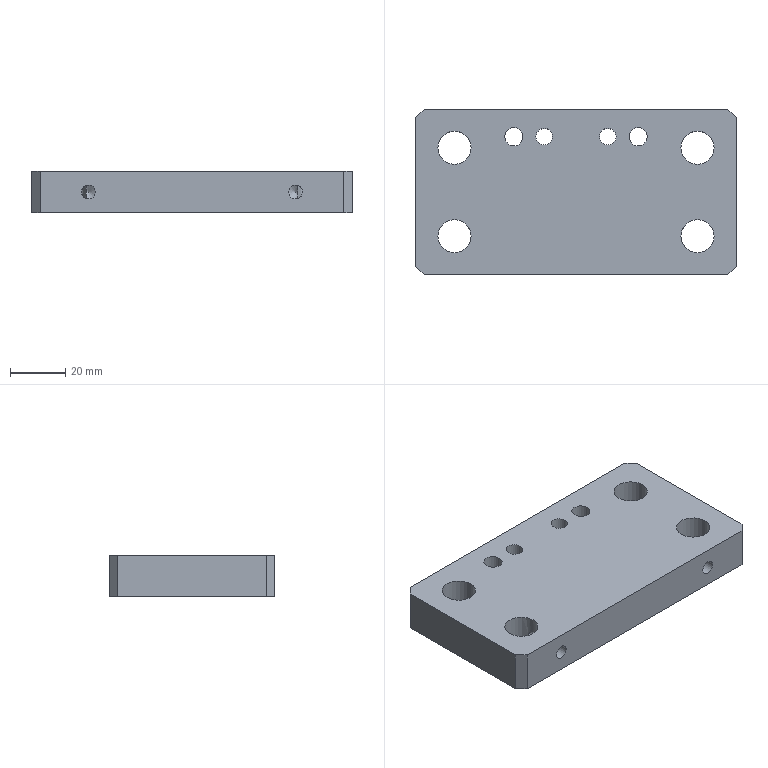Part | NX | features BREP 1 | 1 solid | 29 faces | box 116 x 60 x 15 mm | volume 93839 mm3 | cylinder 14 | plane 12 | cone 3 | commonest cylinder face diameters 5 x4 12 x4 6 x2 6.6 x2 11 x2
STEP:
#1=CARTESIAN_POINT('',(58.,0.,-5.));
#2=VERTEX_POINT('',#1);
#3=CARTESIAN_POINT('',(58.,0.,-7.5));
#4=DIRECTION('',(-1.,0.,0.));
#5=DIRECTION('',(0.,0.,1.));
#6=AXIS2_PLACEMENT_3D('',#3,#4,#5);
#7=CIRCLE('',#6,2.5);
#8=EDGE_CURVE('',#2,#2,#7,.T.);
#9=ORIENTED_EDGE('',*,*,#8,.T.);
#10=EDGE_LOOP('',(#9));
#11=FACE_BOUND('',#10,.T.);
#12=CARTESIAN_POINT('',(58.,-27.,0.));
#13=VERTEX_POINT('',#12);
#14=CARTESIAN_POINT('',(58.,27.,0.));
#15=VERTEX_POINT('',#14);
#16=CARTESIAN_POINT('',(58.,30.,0.));
#17=DIRECTION('',(0.,1.,0.));
#18=VECTOR('',#17,1000.);
#19=LINE('',#16,#18);
#20=EDGE_CURVE('',#13,#15,#19,.T.);
#21=ORIENTED_EDGE('',*,*,#20,.F.);
#22=CARTESIAN_POINT('',(58.,-27.,-15.));
#23=VERTEX_POINT('',#22);
#24=CARTESIAN_POINT('',(58.,-27.,-15.));
#25=DIRECTION('',(0.,0.,1.));
#26=VECTOR('',#25,1000.);
#27=LINE('',#24,#26);
#28=EDGE_CURVE('',#23,#13,#27,.T.);
#29=ORIENTED_EDGE('',*,*,#28,.F.);
#30=CARTESIAN_POINT('',(58.,27.,-15.));
#31=VERTEX_POINT('',#30);
#32=CARTESIAN_POINT('',(58.,30.,-15.));
#33=DIRECTION('',(0.,1.,0.));
#34=VECTOR('',#33,1000.);
#35=LINE('',#32,#34);
#36=EDGE_CURVE('',#23,#31,#35,.T.);
#37=ORIENTED_EDGE('',*,*,#36,.T.);
#38=CARTESIAN_POINT('',(58.,27.,-15.));
#39=DIRECTION('',(0.,0.,-1.));
#40=VECTOR('',#39,1000.);
#41=LINE('',#38,#40);
#42=EDGE_CURVE('',#15,#31,#41,.T.);
#43=ORIENTED_EDGE('',*,*,#42,.F.);
#44=EDGE_LOOP('',(#21,#29,#37,#43));
#45=FACE_BOUND('',#44,.T.);
#46=CARTESIAN_POINT('',(58.,30.,-15.));
#47=DIRECTION('',(-1.,0.,0.));
#48=DIRECTION('',(0.,1.,0.));
#49=AXIS2_PLACEMENT_3D('',#46,#47,#48);
#50=PLANE('',#49);
#51=ADVANCED_FACE('',(#11,#45),#50,.F.);
#52=CARTESIAN_POINT('',(55.,30.,-15.));
#53=VERTEX_POINT('',#52);
#54=CARTESIAN_POINT('',(-55.,30.,-15.));
#55=VERTEX_POINT('',#54);
#56=CARTESIAN_POINT('',(-58.,30.,-15.));
#57=DIRECTION('',(-1.,0.,0.));
#58=VECTOR('',#57,1000.);
#59=LINE('',#56,#58);
#60=EDGE_CURVE('',#53,#55,#59,.T.);
#61=ORIENTED_EDGE('',*,*,#60,.T.);
#62=CARTESIAN_POINT('',(-55.,30.,0.));
#63=VERTEX_POINT('',#62);
#64=CARTESIAN_POINT('',(-55.,30.,-15.));
#65=DIRECTION('',(0.,0.,-1.));
#66=VECTOR('',#65,1000.);
#67=LINE('',#64,#66);
#68=EDGE_CURVE('',#63,#55,#67,.T.);
#69=ORIENTED_EDGE('',*,*,#68,.F.);
#70=CARTESIAN_POINT('',(55.,30.,0.));
#71=VERTEX_POINT('',#70);
#72=CARTESIAN_POINT('',(-58.,30.,0.));
#73=DIRECTION('',(-1.,0.,0.));
#74=VECTOR('',#73,1000.);
#75=LINE('',#72,#74);
#76=EDGE_CURVE('',#71,#63,#75,.T.);
#77=ORIENTED_EDGE('',*,*,#76,.F.);
#78=CARTESIAN_POINT('',(55.,30.,-15.));
#79=DIRECTION('',(0.,0.,1.));
#80=VECTOR('',#79,1000.);
#81=LINE('',#78,#80);
#82=EDGE_CURVE('',#53,#71,#81,.T.);
#83=ORIENTED_EDGE('',*,*,#82,.F.);
#84=EDGE_LOOP('',(#61,#69,#77,#83));
#85=FACE_BOUND('',#84,.T.);
#86=CARTESIAN_POINT('',(-58.,30.,-15.));
#87=DIRECTION('',(0.,-1.,0.));
#88=DIRECTION('',(0.,0.,-1.));
#89=AXIS2_PLACEMENT_3D('',#86,#87,#88);
#90=PLANE('',#89);
#91=ADVANCED_FACE('',(#85),#90,.F.);
#92=CARTESIAN_POINT('',(-58.,27.,-15.));
#93=VERTEX_POINT('',#92);
#94=CARTESIAN_POINT('',(-58.,-27.,-15.));
#95=VERTEX_POINT('',#94);
#96=CARTESIAN_POINT('',(-58.,30.,-15.));
#97=DIRECTION('',(0.,-1.,0.));
#98=VECTOR('',#97,1000.);
#99=LINE('',#96,#98);
#100=EDGE_CURVE('',#93,#95,#99,.T.);
#101=ORIENTED_EDGE('',*,*,#100,.T.);
#102=CARTESIAN_POINT('',(-58.,-27.,0.));
#103=VERTEX_POINT('',#102);
#104=CARTESIAN_POINT('',(-58.,-27.,-15.));
#105=DIRECTION('',(0.,0.,-1.));
#106=VECTOR('',#105,1000.);
#107=LINE('',#104,#106);
#108=EDGE_CURVE('',#103,#95,#107,.T.);
#109=ORIENTED_EDGE('',*,*,#108,.F.);
#110=CARTESIAN_POINT('',(-58.,27.,0.));
#111=VERTEX_POINT('',#110);
#112=CARTESIAN_POINT('',(-58.,30.,0.));
#113=DIRECTION('',(0.,-1.,0.));
#114=VECTOR('',#113,1000.);
#115=LINE('',#112,#114);
#116=EDGE_CURVE('',#111,#103,#115,.T.);
#117=ORIENTED_EDGE('',*,*,#116,.F.);
#118=CARTESIAN_POINT('',(-58.,27.,-15.));
#119=DIRECTION('',(0.,0.,1.));
#120=VECTOR('',#119,1000.);
#121=LINE('',#118,#120);
#122=EDGE_CURVE('',#93,#111,#121,.T.);
#123=ORIENTED_EDGE('',*,*,#122,.F.);
#124=EDGE_LOOP('',(#101,#109,#117,#123));
#125=FACE_BOUND('',#124,.T.);
#126=CARTESIAN_POINT('',(-58.,30.,-15.));
#127=DIRECTION('',(1.,0.,0.));
#128=DIRECTION('',(0.,-1.,0.));
#129=AXIS2_PLACEMENT_3D('',#126,#127,#128);
#130=PLANE('',#129);
#131=ADVANCED_FACE('',(#125),#130,.F.);
#132=CARTESIAN_POINT('',(37.5,-30.,-5.));
#133=VERTEX_POINT('',#132);
#134=CARTESIAN_POINT('',(37.5,-30.,-7.5));
#135=DIRECTION('',(0.,1.,0.));
#136=DIRECTION('',(0.,0.,1.));
#137=AXIS2_PLACEMENT_3D('',#134,#135,#136);
#138=CIRCLE('',#137,2.5);
#139=EDGE_CURVE('',#133,#133,#138,.T.);
#140=ORIENTED_EDGE('',*,*,#139,.T.);
#141=EDGE_LOOP('',(#140));
#142=FACE_BOUND('',#141,.T.);
#143=CARTESIAN_POINT('',(-37.5,-30.,-5.));
#144=VERTEX_POINT('',#143);
#145=CARTESIAN_POINT('',(-37.5,-30.,-7.5));
#146=DIRECTION('',(0.,1.,0.));
#147=DIRECTION('',(0.,0.,1.));
#148=AXIS2_PLACEMENT_3D('',#145,#146,#147);
#149=CIRCLE('',#148,2.5);
#150=EDGE_CURVE('',#144,#144,#149,.T.);
#151=ORIENTED_EDGE('',*,*,#150,.T.);
#152=EDGE_LOOP('',(#151));
#153=FACE_BOUND('',#152,.T.);
#154=CARTESIAN_POINT('',(-55.,-30.,0.));
#155=VERTEX_POINT('',#154);
#156=CARTESIAN_POINT('',(55.,-30.,0.));
#157=VERTEX_POINT('',#156);
#158=CARTESIAN_POINT('',(-58.,-30.,0.));
#159=DIRECTION('',(1.,0.,0.));
#160=VECTOR('',#159,1000.);
#161=LINE('',#158,#160);
#162=EDGE_CURVE('',#155,#157,#161,.T.);
#163=ORIENTED_EDGE('',*,*,#162,.F.);
#164=CARTESIAN_POINT('',(-55.,-30.,-15.));
#165=VERTEX_POINT('',#164);
#166=CARTESIAN_POINT('',(-55.,-30.,-15.));
#167=DIRECTION('',(0.,0.,1.));
#168=VECTOR('',#167,1000.);
#169=LINE('',#166,#168);
#170=EDGE_CURVE('',#165,#155,#169,.T.);
#171=ORIENTED_EDGE('',*,*,#170,.F.);
#172=CARTESIAN_POINT('',(55.,-30.,-15.));
#173=VERTEX_POINT('',#172);
#174=CARTESIAN_POINT('',(-58.,-30.,-15.));
#175=DIRECTION('',(1.,0.,0.));
#176=VECTOR('',#175,1000.);
#177=LINE('',#174,#176);
#178=EDGE_CURVE('',#165,#173,#177,.T.);
#179=ORIENTED_EDGE('',*,*,#178,.T.);
#180=CARTESIAN_POINT('',(55.,-30.,-15.));
#181=DIRECTION('',(0.,0.,-1.));
#182=VECTOR('',#181,1000.);
#183=LINE('',#180,#182);
#184=EDGE_CURVE('',#157,#173,#183,.T.);
#185=ORIENTED_EDGE('',*,*,#184,.F.);
#186=EDGE_LOOP('',(#163,#171,#179,#185));
#187=FACE_BOUND('',#186,.T.);
#188=CARTESIAN_POINT('',(-58.,-30.,-15.));
#189=DIRECTION('',(0.,1.,0.));
#190=DIRECTION('',(0.,0.,1.));
#191=AXIS2_PLACEMENT_3D('',#188,#189,#190);
#192=PLANE('',#191);
#193=ADVANCED_FACE('',(#142,#153,#187),#192,.F.);
#194=CARTESIAN_POINT('',(38.,16.,-15.));
#195=VERTEX_POINT('',#194);
#196=CARTESIAN_POINT('',(44.,16.,-15.));
#197=DIRECTION('',(0.,0.,-1.));
#198=DIRECTION('',(-1.,0.,0.));
#199=AXIS2_PLACEMENT_3D('',#196,#197,#198);
#200=CIRCLE('',#199,6.);
#201=EDGE_CURVE('',#195,#195,#200,.T.);
#202=ORIENTED_EDGE('',*,*,#201,.F.);
#203=EDGE_LOOP('',(#202));
#204=FACE_BOUND('',#203,.T.);
#205=CARTESIAN_POINT('',(38.,-16.,-15.));
#206=VERTEX_POINT('',#205);
#207=CARTESIAN_POINT('',(44.,-16.,-15.));
#208=DIRECTION('',(0.,0.,-1.));
#209=DIRECTION('',(-1.,0.,0.));
#210=AXIS2_PLACEMENT_3D('',#207,#208,#209);
#211=CIRCLE('',#210,6.);
#212=EDGE_CURVE('',#206,#206,#211,.T.);
#213=ORIENTED_EDGE('',*,*,#212,.F.);
#214=EDGE_LOOP('',(#213));
#215=FACE_BOUND('',#214,.T.);
#216=CARTESIAN_POINT('',(-50.,-16.,-15.));
#217=VERTEX_POINT('',#216);
#218=CARTESIAN_POINT('',(-44.,-16.,-15.));
#219=DIRECTION('',(0.,0.,-1.));
#220=DIRECTION('',(-1.,0.,0.));
#221=AXIS2_PLACEMENT_3D('',#218,#219,#220);
#222=CIRCLE('',#221,6.);
#223=EDGE_CURVE('',#217,#217,#222,.T.);
#224=ORIENTED_EDGE('',*,*,#223,.F.);
#225=EDGE_LOOP('',(#224));
#226=FACE_BOUND('',#225,.T.);
#227=CARTESIAN_POINT('',(-50.,16.,-15.));
#228=VERTEX_POINT('',#227);
#229=CARTESIAN_POINT('',(-44.,16.,-15.));
#230=DIRECTION('',(0.,0.,-1.));
#231=DIRECTION('',(-1.,0.,0.));
#232=AXIS2_PLACEMENT_3D('',#229,#230,#231);
#233=CIRCLE('',#232,6.);
#234=EDGE_CURVE('',#228,#228,#233,.T.);
#235=ORIENTED_EDGE('',*,*,#234,.F.);
#236=EDGE_LOOP('',(#235));
#237=FACE_BOUND('',#236,.T.);
#238=CARTESIAN_POINT('',(28.,20.,-15.));
#239=VERTEX_POINT('',#238);
#240=CARTESIAN_POINT('',(22.5,20.,-15.));
#241=DIRECTION('',(0.,0.,1.));
#242=DIRECTION('',(1.,0.,0.));
#243=AXIS2_PLACEMENT_3D('',#240,#241,#242);
#244=CIRCLE('',#243,5.5);
#245=EDGE_CURVE('',#239,#239,#244,.T.);
#246=ORIENTED_EDGE('',*,*,#245,.T.);
#247=EDGE_LOOP('',(#246));
#248=FACE_BOUND('',#247,.T.);
#249=CARTESIAN_POINT('',(-17.,20.,-15.));
#250=VERTEX_POINT('',#249);
#251=CARTESIAN_POINT('',(-22.5,20.,-15.));
#252=DIRECTION('',(0.,0.,1.));
#253=DIRECTION('',(1.,0.,0.));
#254=AXIS2_PLACEMENT_3D('',#251,#252,#253);
#255=CIRCLE('',#254,5.5);
#256=EDGE_CURVE('',#250,#250,#255,.T.);
#257=ORIENTED_EDGE('',*,*,#256,.T.);
#258=EDGE_LOOP('',(#257));
#259=FACE_BOUND('',#258,.T.);
#260=CARTESIAN_POINT('',(-14.5,20.,-15.));
#261=VERTEX_POINT('',#260);
#262=CARTESIAN_POINT('',(-11.5,20.,-15.));
#263=DIRECTION('',(0.,0.,-1.));
#264=DIRECTION('',(-1.,0.,0.));
#265=AXIS2_PLACEMENT_3D('',#262,#263,#264);
#266=CIRCLE('',#265,3.);
#267=EDGE_CURVE('',#261,#261,#266,.T.);
#268=ORIENTED_EDGE('',*,*,#267,.F.);
#269=EDGE_LOOP('',(#268));
#270=FACE_BOUND('',#269,.T.);
#271=CARTESIAN_POINT('',(8.5,20.,-15.));
#272=VERTEX_POINT('',#271);
#273=CARTESIAN_POINT('',(11.5,20.,-15.));
#274=DIRECTION('',(0.,0.,-1.));
#275=DIRECTION('',(-1.,0.,0.));
#276=AXIS2_PLACEMENT_3D('',#273,#274,#275);
#277=CIRCLE('',#276,3.);
#278=EDGE_CURVE('',#272,#272,#277,.T.);
#279=ORIENTED_EDGE('',*,*,#278,.F.);
#280=EDGE_LOOP('',(#279));
#281=FACE_BOUND('',#280,.T.);
#282=ORIENTED_EDGE('',*,*,#36,.F.);
#283=CARTESIAN_POINT('',(42.5,-42.5,-15.));
#284=DIRECTION('',(0.7071,0.7071,0.));
#285=VECTOR('',#284,1000.);
#286=LINE('',#283,#285);
#287=EDGE_CURVE('',#173,#23,#286,.T.);
#288=ORIENTED_EDGE('',*,*,#287,.F.);
#289=ORIENTED_EDGE('',*,*,#178,.F.);
#290=CARTESIAN_POINT('',(-42.5,-42.5,-15.));
#291=DIRECTION('',(0.7071,-0.7071,0.));
#292=VECTOR('',#291,1000.);
#293=LINE('',#290,#292);
#294=EDGE_CURVE('',#95,#165,#293,.T.);
#295=ORIENTED_EDGE('',*,*,#294,.F.);
#296=ORIENTED_EDGE('',*,*,#100,.F.);
#297=CARTESIAN_POINT('',(-42.5,42.5,-15.));
#298=DIRECTION('',(-0.7071,-0.7071,0.));
#299=VECTOR('',#298,1000.);
#300=LINE('',#297,#299);
#301=EDGE_CURVE('',#55,#93,#300,.T.);
#302=ORIENTED_EDGE('',*,*,#301,.F.);
#303=ORIENTED_EDGE('',*,*,#60,.F.);
#304=CARTESIAN_POINT('',(42.5,42.5,-15.));
#305=DIRECTION('',(-0.7071,0.7071,0.));
#306=VECTOR('',#305,1000.);
#307=LINE('',#304,#306);
#308=EDGE_CURVE('',#31,#53,#307,.T.);
#309=ORIENTED_EDGE('',*,*,#308,.F.);
#310=EDGE_LOOP('',(#282,#288,#289,#295,#296,#302,#303,#309));
#311=FACE_BOUND('',#310,.T.);
#312=CARTESIAN_POINT('',(0.,0.,-15.));
#313=DIRECTION('',(0.,0.,-1.));
#314=DIRECTION('',(-1.,0.,0.));
#315=AXIS2_PLACEMENT_3D('',#312,#313,#314);
#316=PLANE('',#315);
#317=ADVANCED_FACE('',(#204,#215,#226,#237,#248,#259,#270,#281,#311),#316,.T.);
#318=CARTESIAN_POINT('',(38.,16.,0.));
#319=VERTEX_POINT('',#318);
#320=CARTESIAN_POINT('',(44.,16.,0.));
#321=DIRECTION('',(0.,0.,-1.));
#322=DIRECTION('',(-1.,0.,0.));
#323=AXIS2_PLACEMENT_3D('',#320,#321,#322);
#324=CIRCLE('',#323,6.);
#325=EDGE_CURVE('',#319,#319,#324,.T.);
#326=ORIENTED_EDGE('',*,*,#325,.T.);
#327=EDGE_LOOP('',(#326));
#328=FACE_BOUND('',#327,.T.);
#329=CARTESIAN_POINT('',(38.,-16.,0.));
#330=VERTEX_POINT('',#329);
#331=CARTESIAN_POINT('',(44.,-16.,0.));
#332=DIRECTION('',(0.,0.,-1.));
#333=DIRECTION('',(-1.,0.,0.));
#334=AXIS2_PLACEMENT_3D('',#331,#332,#333);
#335=CIRCLE('',#334,6.);
#336=EDGE_CURVE('',#330,#330,#335,.T.);
#337=ORIENTED_EDGE('',*,*,#336,.T.);
#338=EDGE_LOOP('',(#337));
#339=FACE_BOUND('',#338,.T.);
#340=CARTESIAN_POINT('',(-50.,-16.,0.));
#341=VERTEX_POINT('',#340);
#342=CARTESIAN_POINT('',(-44.,-16.,0.));
#343=DIRECTION('',(0.,0.,-1.));
#344=DIRECTION('',(-1.,0.,0.));
#345=AXIS2_PLACEMENT_3D('',#342,#343,#344);
#346=CIRCLE('',#345,6.);
#347=EDGE_CURVE('',#341,#341,#346,.T.);
#348=ORIENTED_EDGE('',*,*,#347,.T.);
#349=EDGE_LOOP('',(#348));
#350=FACE_BOUND('',#349,.T.);
#351=CARTESIAN_POINT('',(-50.,16.,0.));
#352=VERTEX_POINT('',#351);
#353=CARTESIAN_POINT('',(-44.,16.,0.));
#354=DIRECTION('',(0.,0.,-1.));
#355=DIRECTION('',(-1.,0.,0.));
#356=AXIS2_PLACEMENT_3D('',#353,#354,#355);
#357=CIRCLE('',#356,6.);
#358=EDGE_CURVE('',#352,#352,#357,.T.);
#359=ORIENTED_EDGE('',*,*,#358,.T.);
#360=EDGE_LOOP('',(#359));
#361=FACE_BOUND('',#360,.T.);
#362=CARTESIAN_POINT('',(25.8,20.,0.));
#363=VERTEX_POINT('',#362);
#364=CARTESIAN_POINT('',(22.5,20.,0.));
#365=DIRECTION('',(0.,0.,1.));
#366=DIRECTION('',(1.,0.,0.));
#367=AXIS2_PLACEMENT_3D('',#364,#365,#366);
#368=CIRCLE('',#367,3.3);
#369=EDGE_CURVE('',#363,#363,#368,.T.);
#370=ORIENTED_EDGE('',*,*,#369,.F.);
#371=EDGE_LOOP('',(#370));
#372=FACE_BOUND('',#371,.T.);
#373=CARTESIAN_POINT('',(-19.2,20.,0.));
#374=VERTEX_POINT('',#373);
#375=CARTESIAN_POINT('',(-22.5,20.,0.));
#376=DIRECTION('',(0.,0.,1.));
#377=DIRECTION('',(1.,0.,0.));
#378=AXIS2_PLACEMENT_3D('',#375,#376,#377);
#379=CIRCLE('',#378,3.3);
#380=EDGE_CURVE('',#374,#374,#379,.T.);
#381=ORIENTED_EDGE('',*,*,#380,.F.);
#382=EDGE_LOOP('',(#381));
#383=FACE_BOUND('',#382,.T.);
#384=CARTESIAN_POINT('',(-14.5,20.,0.));
#385=VERTEX_POINT('',#384);
#386=CARTESIAN_POINT('',(-11.5,20.,0.));
#387=DIRECTION('',(0.,0.,-1.));
#388=DIRECTION('',(-1.,0.,0.));
#389=AXIS2_PLACEMENT_3D('',#386,#387,#388);
#390=CIRCLE('',#389,3.);
#391=EDGE_CURVE('',#385,#385,#390,.T.);
#392=ORIENTED_EDGE('',*,*,#391,.T.);
#393=EDGE_LOOP('',(#392));
#394=FACE_BOUND('',#393,.T.);
#395=CARTESIAN_POINT('',(8.5,20.,0.));
#396=VERTEX_POINT('',#395);
#397=CARTESIAN_POINT('',(11.5,20.,0.));
#398=DIRECTION('',(0.,0.,-1.));
#399=DIRECTION('',(-1.,0.,0.));
#400=AXIS2_PLACEMENT_3D('',#397,#398,#399);
#401=CIRCLE('',#400,3.);
#402=EDGE_CURVE('',#396,#396,#401,.T.);
#403=ORIENTED_EDGE('',*,*,#402,.T.);
#404=EDGE_LOOP('',(#403));
#405=FACE_BOUND('',#404,.T.);
#406=ORIENTED_EDGE('',*,*,#76,.T.);
#407=CARTESIAN_POINT('',(-58.,27.,0.));
#408=DIRECTION('',(0.7071,0.7071,0.));
#409=VECTOR('',#408,1000.);
#410=LINE('',#407,#409);
#411=EDGE_CURVE('',#111,#63,#410,.T.);
#412=ORIENTED_EDGE('',*,*,#411,.F.);
#413=ORIENTED_EDGE('',*,*,#116,.T.);
#414=CARTESIAN_POINT('',(-55.,-30.,0.));
#415=DIRECTION('',(-0.7071,0.7071,0.));
#416=VECTOR('',#415,1000.);
#417=LINE('',#414,#416);
#418=EDGE_CURVE('',#155,#103,#417,.T.);
#419=ORIENTED_EDGE('',*,*,#418,.F.);
#420=ORIENTED_EDGE('',*,*,#162,.T.);
#421=CARTESIAN_POINT('',(58.,-27.,0.));
#422=DIRECTION('',(-0.7071,-0.7071,0.));
#423=VECTOR('',#422,1000.);
#424=LINE('',#421,#423);
#425=EDGE_CURVE('',#13,#157,#424,.T.);
#426=ORIENTED_EDGE('',*,*,#425,.F.);
#427=ORIENTED_EDGE('',*,*,#20,.T.);
#428=CARTESIAN_POINT('',(55.,30.,0.));
#429=DIRECTION('',(0.7071,-0.7071,0.));
#430=VECTOR('',#429,1000.);
#431=LINE('',#428,#430);
#432=EDGE_CURVE('',#71,#15,#431,.T.);
#433=ORIENTED_EDGE('',*,*,#432,.F.);
#434=EDGE_LOOP('',(#406,#412,#413,#419,#420,#426,#427,#433));
#435=FACE_BOUND('',#434,.T.);
#436=CARTESIAN_POINT('',(0.,0.,0.));
#437=DIRECTION('',(0.,0.,-1.));
#438=DIRECTION('',(-1.,0.,0.));
#439=AXIS2_PLACEMENT_3D('',#436,#437,#438);
#440=PLANE('',#439);
#441=ADVANCED_FACE('',(#328,#339,#350,#361,#372,#383,#394,#405,#435),#440,.F.);
#442=ORIENTED_EDGE('',*,*,#278,.T.);
#443=EDGE_LOOP('',(#442));
#444=FACE_BOUND('',#443,.T.);
#445=ORIENTED_EDGE('',*,*,#402,.F.);
#446=EDGE_LOOP('',(#445));
#447=FACE_BOUND('',#446,.T.);
#448=CARTESIAN_POINT('',(11.5,20.,0.));
#449=DIRECTION('',(0.,0.,1.));
#450=DIRECTION('',(1.,0.,0.));
#451=AXIS2_PLACEMENT_3D('',#448,#449,#450);
#452=CYLINDRICAL_SURFACE('',#451,3.);
#453=ADVANCED_FACE('',(#444,#447),#452,.F.);
#454=ORIENTED_EDGE('',*,*,#267,.T.);
#455=EDGE_LOOP('',(#454));
#456=FACE_BOUND('',#455,.T.);
#457=ORIENTED_EDGE('',*,*,#391,.F.);
#458=EDGE_LOOP('',(#457));
#459=FACE_BOUND('',#458,.T.);
#460=CARTESIAN_POINT('',(-11.5,20.,0.));
#461=DIRECTION('',(0.,0.,1.));
#462=DIRECTION('',(1.,0.,0.));
#463=AXIS2_PLACEMENT_3D('',#460,#461,#462);
#464=CYLINDRICAL_SURFACE('',#463,3.);
#465=ADVANCED_FACE('',(#456,#459),#464,.F.);
#466=ORIENTED_EDGE('',*,*,#380,.T.);
#467=EDGE_LOOP('',(#466));
#468=FACE_BOUND('',#467,.T.);
#469=CARTESIAN_POINT('',(-19.2,20.,-8.6));
#470=VERTEX_POINT('',#469);
#471=CARTESIAN_POINT('',(-22.5,20.,-8.6));
#472=DIRECTION('',(0.,0.,1.));
#473=DIRECTION('',(1.,0.,0.));
#474=AXIS2_PLACEMENT_3D('',#471,#472,#473);
#475=CIRCLE('',#474,3.3);
#476=EDGE_CURVE('',#470,#470,#475,.T.);
#477=ORIENTED_EDGE('',*,*,#476,.F.);
#478=EDGE_LOOP('',(#477));
#479=FACE_BOUND('',#478,.T.);
#480=CARTESIAN_POINT('',(-22.5,20.,-15.));
#481=DIRECTION('',(0.,0.,-1.));
#482=DIRECTION('',(-1.,0.,0.));
#483=AXIS2_PLACEMENT_3D('',#480,#481,#482);
#484=CYLINDRICAL_SURFACE('',#483,3.3);
#485=ADVANCED_FACE('',(#468,#479),#484,.F.);
#486=ORIENTED_EDGE('',*,*,#476,.T.);
#487=EDGE_LOOP('',(#486));
#488=FACE_BOUND('',#487,.T.);
#489=CARTESIAN_POINT('',(-17.,20.,-8.6));
#490=VERTEX_POINT('',#489);
#491=CARTESIAN_POINT('',(-22.5,20.,-8.6));
#492=DIRECTION('',(0.,0.,1.));
#493=DIRECTION('',(1.,0.,0.));
#494=AXIS2_PLACEMENT_3D('',#491,#492,#493);
#495=CIRCLE('',#494,5.5);
#496=EDGE_CURVE('',#490,#490,#495,.T.);
#497=ORIENTED_EDGE('',*,*,#496,.F.);
#498=EDGE_LOOP('',(#497));
#499=FACE_BOUND('',#498,.T.);
#500=CARTESIAN_POINT('',(-19.2,20.,-8.6));
#501=DIRECTION('',(0.,0.,1.));
#502=DIRECTION('',(1.,0.,0.));
#503=AXIS2_PLACEMENT_3D('',#500,#501,#502);
#504=PLANE('',#503);
#505=ADVANCED_FACE('',(#488,#499),#504,.F.);
#506=ORIENTED_EDGE('',*,*,#496,.T.);
#507=EDGE_LOOP('',(#506));
#508=FACE_BOUND('',#507,.T.);
#509=ORIENTED_EDGE('',*,*,#256,.F.);
#510=EDGE_LOOP('',(#509));
#511=FACE_BOUND('',#510,.T.);
#512=CARTESIAN_POINT('',(-22.5,20.,-15.));
#513=DIRECTION('',(0.,0.,-1.));
#514=DIRECTION('',(-1.,0.,0.));
#515=AXIS2_PLACEMENT_3D('',#512,#513,#514);
#516=CYLINDRICAL_SURFACE('',#515,5.5);
#517=ADVANCED_FACE('',(#508,#511),#516,.F.);
#518=ORIENTED_EDGE('',*,*,#369,.T.);
#519=EDGE_LOOP('',(#518));
#520=FACE_BOUND('',#519,.T.);
#521=CARTESIAN_POINT('',(25.8,20.,-8.6));
#522=VERTEX_POINT('',#521);
#523=CARTESIAN_POINT('',(22.5,20.,-8.6));
#524=DIRECTION('',(0.,0.,1.));
#525=DIRECTION('',(1.,0.,0.));
#526=AXIS2_PLACEMENT_3D('',#523,#524,#525);
#527=CIRCLE('',#526,3.3);
#528=EDGE_CURVE('',#522,#522,#527,.T.);
#529=ORIENTED_EDGE('',*,*,#528,.F.);
#530=EDGE_LOOP('',(#529));
#531=FACE_BOUND('',#530,.T.);
#532=CARTESIAN_POINT('',(22.5,20.,-15.));
#533=DIRECTION('',(0.,0.,-1.));
#534=DIRECTION('',(-1.,0.,0.));
#535=AXIS2_PLACEMENT_3D('',#532,#533,#534);
#536=CYLINDRICAL_SURFACE('',#535,3.3);
#537=ADVANCED_FACE('',(#520,#531),#536,.F.);
#538=ORIENTED_EDGE('',*,*,#528,.T.);
#539=EDGE_LOOP('',(#538));
#540=FACE_BOUND('',#539,.T.);
#541=CARTESIAN_POINT('',(28.,20.,-8.6));
#542=VERTEX_POINT('',#541);
#543=CARTESIAN_POINT('',(22.5,20.,-8.6));
#544=DIRECTION('',(0.,0.,1.));
#545=DIRECTION('',(1.,0.,0.));
#546=AXIS2_PLACEMENT_3D('',#543,#544,#545);
#547=CIRCLE('',#546,5.5);
#548=EDGE_CURVE('',#542,#542,#547,.T.);
#549=ORIENTED_EDGE('',*,*,#548,.F.);
#550=EDGE_LOOP('',(#549));
#551=FACE_BOUND('',#550,.T.);
#552=CARTESIAN_POINT('',(25.8,20.,-8.6));
#553=DIRECTION('',(0.,0.,1.));
#554=DIRECTION('',(1.,0.,0.));
#555=AXIS2_PLACEMENT_3D('',#552,#553,#554);
#556=PLANE('',#555);
#557=ADVANCED_FACE('',(#540,#551),#556,.F.);
#558=ORIENTED_EDGE('',*,*,#548,.T.);
#559=EDGE_LOOP('',(#558));
#560=FACE_BOUND('',#559,.T.);
#561=ORIENTED_EDGE('',*,*,#245,.F.);
#562=EDGE_LOOP('',(#561));
#563=FACE_BOUND('',#562,.T.);
#564=CARTESIAN_POINT('',(22.5,20.,-15.));
#565=DIRECTION('',(0.,0.,-1.));
#566=DIRECTION('',(-1.,0.,0.));
#567=AXIS2_PLACEMENT_3D('',#564,#565,#566);
#568=CYLINDRICAL_SURFACE('',#567,5.5);
#569=ADVANCED_FACE('',(#560,#563),#568,.F.);
#570=ORIENTED_EDGE('',*,*,#234,.T.);
#571=EDGE_LOOP('',(#570));
#572=FACE_BOUND('',#571,.T.);
#573=ORIENTED_EDGE('',*,*,#358,.F.);
#574=EDGE_LOOP('',(#573));
#575=FACE_BOUND('',#574,.T.);
#576=CARTESIAN_POINT('',(-44.,16.,0.));
#577=DIRECTION('',(0.,0.,1.));
#578=DIRECTION('',(1.,0.,0.));
#579=AXIS2_PLACEMENT_3D('',#576,#577,#578);
#580=CYLINDRICAL_SURFACE('',#579,6.);
#581=ADVANCED_FACE('',(#572,#575),#580,.F.);
#582=CARTESIAN_POINT('',(-38.084,-15.,-9.931));
#583=VERTEX_POINT('',#582);
#584=CARTESIAN_POINT('',(-38.084,-15.,-5.069));
#585=VERTEX_POINT('',#584);
#586=CARTESIAN_POINT('',(-38.084,-15.,-9.931));
#587=CARTESIAN_POINT('',(-37.983,-15.598,-9.955));
#588=CARTESIAN_POINT('',(-37.966,-16.805,-9.957));
#589=CARTESIAN_POINT('',(-38.461,-18.547,-9.846));
#590=CARTESIAN_POINT('',(-39.481,-20.042,-9.275));
#591=CARTESIAN_POINT('',(-40.257,-20.685,-7.513));
#592=CARTESIAN_POINT('',(-39.492,-20.053,-5.735));
#593=CARTESIAN_POINT('',(-38.471,-18.568,-5.157));
#594=CARTESIAN_POINT('',(-37.966,-16.82,-5.043));
#595=CARTESIAN_POINT('',(-37.983,-15.598,-5.045));
#596=CARTESIAN_POINT('',(-38.084,-15.,-5.069));
#597=B_SPLINE_CURVE_WITH_KNOTS('',3,(#586,#587,#588,#589,#590,#591,#592,#593,#594,#595,#596),.UNSPECIFIED.,.F.,.F.,(4,1,1,1,1,1,1,1,4),(0.,0.001794,0.003588,0.005381,0.007175,0.008969,0.01076,0.01256,0.01435),.UNSPECIFIED.);
#598=EDGE_CURVE('',#583,#585,#597,.T.);
#599=ORIENTED_EDGE('',*,*,#598,.F.);
#600=CARTESIAN_POINT('',(-38.084,-15.,-5.069));
#601=CARTESIAN_POINT('',(-38.121,-14.78,-5.455));
#602=CARTESIAN_POINT('',(-38.219,-14.353,-6.213));
#603=CARTESIAN_POINT('',(-38.404,-13.829,-7.503));
#604=CARTESIAN_POINT('',(-38.218,-14.355,-8.789));
#605=CARTESIAN_POINT('',(-38.121,-14.781,-9.546));
#606=CARTESIAN_POINT('',(-38.084,-15.,-9.931));
#607=B_SPLINE_CURVE_WITH_KNOTS('',3,(#600,#601,#602,#603,#604,#605,#606),.UNSPECIFIED.,.F.,.F.,(4,1,1,1,4),(0.,0.001335,0.002669,0.004004,0.005339),.UNSPECIFIED.);
#608=EDGE_CURVE('',#585,#583,#607,.T.);
#609=ORIENTED_EDGE('',*,*,#608,.F.);
#610=EDGE_LOOP('',(#599,#609));
#611=FACE_BOUND('',#610,.T.);
#612=ORIENTED_EDGE('',*,*,#223,.T.);
#613=EDGE_LOOP('',(#612));
#614=FACE_BOUND('',#613,.T.);
#615=ORIENTED_EDGE('',*,*,#347,.F.);
#616=EDGE_LOOP('',(#615));
#617=FACE_BOUND('',#616,.T.);
#618=CARTESIAN_POINT('',(-44.,-16.,0.));
#619=DIRECTION('',(0.,0.,1.));
#620=DIRECTION('',(1.,0.,0.));
#621=AXIS2_PLACEMENT_3D('',#618,#619,#620);
#622=CYLINDRICAL_SURFACE('',#621,6.);
#623=ADVANCED_FACE('',(#611,#614,#617),#622,.F.);
#624=CARTESIAN_POINT('',(38.084,-15.,-9.931));
#625=VERTEX_POINT('',#624);
#626=CARTESIAN_POINT('',(38.084,-15.,-5.069));
#627=VERTEX_POINT('',#626);
#628=CARTESIAN_POINT('',(38.084,-15.,-9.931));
#629=CARTESIAN_POINT('',(38.121,-14.78,-9.545));
#630=CARTESIAN_POINT('',(38.219,-14.353,-8.787));
#631=CARTESIAN_POINT('',(38.404,-13.829,-7.497));
#632=CARTESIAN_POINT('',(38.218,-14.355,-6.211));
#633=CARTESIAN_POINT('',(38.121,-14.781,-5.454));
#634=CARTESIAN_POINT('',(38.084,-15.,-5.069));
#635=B_SPLINE_CURVE_WITH_KNOTS('',3,(#628,#629,#630,#631,#632,#633,#634),.UNSPECIFIED.,.F.,.F.,(4,1,1,1,4),(0.,0.001335,0.002669,0.004004,0.005339),.UNSPECIFIED.);
#636=EDGE_CURVE('',#625,#627,#635,.T.);
#637=ORIENTED_EDGE('',*,*,#636,.F.);
#638=CARTESIAN_POINT('',(38.084,-15.,-5.069));
#639=CARTESIAN_POINT('',(37.983,-15.598,-5.045));
#640=CARTESIAN_POINT('',(37.966,-16.805,-5.043));
#641=CARTESIAN_POINT('',(38.461,-18.547,-5.154));
#642=CARTESIAN_POINT('',(39.481,-20.042,-5.725));
#643=CARTESIAN_POINT('',(40.257,-20.685,-7.487));
#644=CARTESIAN_POINT('',(39.492,-20.053,-9.265));
#645=CARTESIAN_POINT('',(38.471,-18.568,-9.843));
#646=CARTESIAN_POINT('',(37.966,-16.82,-9.957));
#647=CARTESIAN_POINT('',(37.983,-15.598,-9.955));
#648=CARTESIAN_POINT('',(38.084,-15.,-9.931));
#649=B_SPLINE_CURVE_WITH_KNOTS('',3,(#638,#639,#640,#641,#642,#643,#644,#645,#646,#647,#648),.UNSPECIFIED.,.F.,.F.,(4,1,1,1,1,1,1,1,4),(0.,0.001794,0.003588,0.005381,0.007175,0.008969,0.01076,0.01256,0.01435),.UNSPECIFIED.);
#650=EDGE_CURVE('',#627,#625,#649,.T.);
#651=ORIENTED_EDGE('',*,*,#650,.F.);
#652=EDGE_LOOP('',(#637,#651));
#653=FACE_BOUND('',#652,.T.);
#654=ORIENTED_EDGE('',*,*,#212,.T.);
#655=EDGE_LOOP('',(#654));
#656=FACE_BOUND('',#655,.T.);
#657=ORIENTED_EDGE('',*,*,#336,.F.);
#658=EDGE_LOOP('',(#657));
#659=FACE_BOUND('',#658,.T.);
#660=CARTESIAN_POINT('',(44.,-16.,0.));
#661=DIRECTION('',(0.,0.,1.));
#662=DIRECTION('',(1.,0.,0.));
#663=AXIS2_PLACEMENT_3D('',#660,#661,#662);
#664=CYLINDRICAL_SURFACE('',#663,6.);
#665=ADVANCED_FACE('',(#653,#656,#659),#664,.F.);
#666=ORIENTED_EDGE('',*,*,#201,.T.);
#667=EDGE_LOOP('',(#666));
#668=FACE_BOUND('',#667,.T.);
#669=ORIENTED_EDGE('',*,*,#325,.F.);
#670=EDGE_LOOP('',(#669));
#671=FACE_BOUND('',#670,.T.);
#672=CARTESIAN_POINT('',(44.,16.,0.));
#673=DIRECTION('',(0.,0.,1.));
#674=DIRECTION('',(1.,0.,0.));
#675=AXIS2_PLACEMENT_3D('',#672,#673,#674);
#676=CYLINDRICAL_SURFACE('',#675,6.);
#677=ADVANCED_FACE('',(#668,#671),#676,.F.);
#678=ORIENTED_EDGE('',*,*,#308,.T.);
#679=ORIENTED_EDGE('',*,*,#82,.T.);
#680=ORIENTED_EDGE('',*,*,#432,.T.);
#681=ORIENTED_EDGE('',*,*,#42,.T.);
#682=EDGE_LOOP('',(#678,#679,#680,#681));
#683=FACE_BOUND('',#682,.T.);
#684=CARTESIAN_POINT('',(55.,30.,-15.));
#685=DIRECTION('',(-0.7071,-0.7071,0.));
#686=DIRECTION('',(0.,0.,-1.));
#687=AXIS2_PLACEMENT_3D('',#684,#685,#686);
#688=PLANE('',#687);
#689=ADVANCED_FACE('',(#683),#688,.F.);
#690=ORIENTED_EDGE('',*,*,#287,.T.);
#691=ORIENTED_EDGE('',*,*,#28,.T.);
#692=ORIENTED_EDGE('',*,*,#425,.T.);
#693=ORIENTED_EDGE('',*,*,#184,.T.);
#694=EDGE_LOOP('',(#690,#691,#692,#693));
#695=FACE_BOUND('',#694,.T.);
#696=CARTESIAN_POINT('',(58.,-27.,-15.));
#697=DIRECTION('',(-0.7071,0.7071,0.));
#698=DIRECTION('',(0.,0.,-1.));
#699=AXIS2_PLACEMENT_3D('',#696,#697,#698);
#700=PLANE('',#699);
#701=ADVANCED_FACE('',(#695),#700,.F.);
#702=ORIENTED_EDGE('',*,*,#301,.T.);
#703=ORIENTED_EDGE('',*,*,#122,.T.);
#704=ORIENTED_EDGE('',*,*,#411,.T.);
#705=ORIENTED_EDGE('',*,*,#68,.T.);
#706=EDGE_LOOP('',(#702,#703,#704,#705));
#707=FACE_BOUND('',#706,.T.);
#708=CARTESIAN_POINT('',(-58.,27.,-15.));
#709=DIRECTION('',(0.7071,-0.7071,0.));
#710=DIRECTION('',(0.,0.,-1.));
#711=AXIS2_PLACEMENT_3D('',#708,#709,#710);
#712=PLANE('',#711);
#713=ADVANCED_FACE('',(#707),#712,.F.);
#714=ORIENTED_EDGE('',*,*,#294,.T.);
#715=ORIENTED_EDGE('',*,*,#170,.T.);
#716=ORIENTED_EDGE('',*,*,#418,.T.);
#717=ORIENTED_EDGE('',*,*,#108,.T.);
#718=EDGE_LOOP('',(#714,#715,#716,#717));
#719=FACE_BOUND('',#718,.T.);
#720=CARTESIAN_POINT('',(-55.,-30.,-15.));
#721=DIRECTION('',(0.7071,0.7071,0.));
#722=DIRECTION('',(0.,0.,-1.));
#723=AXIS2_PLACEMENT_3D('',#720,#721,#722);
#724=PLANE('',#723);
#725=ADVANCED_FACE('',(#719),#724,.F.);
#726=CARTESIAN_POINT('',(-37.5,-15.,-7.5));
#727=DIRECTION('',(0.,1.,0.));
#728=DIRECTION('',(0.,0.,1.));
#729=AXIS2_PLACEMENT_3D('',#726,#727,#728);
#730=CIRCLE('',#729,2.5);
#731=EDGE_CURVE('',#585,#583,#730,.T.);
#732=ORIENTED_EDGE('',*,*,#731,.F.);
#733=ORIENTED_EDGE('',*,*,#608,.T.);
#734=EDGE_LOOP('',(#732,#733));
#735=FACE_BOUND('',#734,.T.);
#736=CARTESIAN_POINT('',(-37.5,-15.,-7.5));
#737=DIRECTION('',(0.,-1.,0.));
#738=DIRECTION('',(0.,0.,-1.));
#739=AXIS2_PLACEMENT_3D('',#736,#737,#738);
#740=CONICAL_SURFACE('',#739,2.5,1.03);
#741=ADVANCED_FACE('',(#735),#740,.F.);
#742=ORIENTED_EDGE('',*,*,#150,.F.);
#743=EDGE_LOOP('',(#742));
#744=FACE_BOUND('',#743,.T.);
#745=ORIENTED_EDGE('',*,*,#731,.T.);
#746=ORIENTED_EDGE('',*,*,#598,.T.);
#747=EDGE_LOOP('',(#745,#746));
#748=FACE_BOUND('',#747,.T.);
#749=CARTESIAN_POINT('',(-37.5,-30.,-7.5));
#750=DIRECTION('',(0.,-1.,0.));
#751=DIRECTION('',(0.,0.,-1.));
#752=AXIS2_PLACEMENT_3D('',#749,#750,#751);
#753=CYLINDRICAL_SURFACE('',#752,2.5);
#754=ADVANCED_FACE('',(#744,#748),#753,.F.);
#755=ORIENTED_EDGE('',*,*,#139,.F.);
#756=EDGE_LOOP('',(#755));
#757=FACE_BOUND('',#756,.T.);
#758=CARTESIAN_POINT('',(37.5,-15.,-7.5));
#759=DIRECTION('',(0.,1.,0.));
#760=DIRECTION('',(0.,0.,1.));
#761=AXIS2_PLACEMENT_3D('',#758,#759,#760);
#762=CIRCLE('',#761,2.5);
#763=EDGE_CURVE('',#625,#627,#762,.T.);
#764=ORIENTED_EDGE('',*,*,#763,.T.);
#765=ORIENTED_EDGE('',*,*,#650,.T.);
#766=EDGE_LOOP('',(#764,#765));
#767=FACE_BOUND('',#766,.T.);
#768=CARTESIAN_POINT('',(37.5,-30.,-7.5));
#769=DIRECTION('',(0.,-1.,0.));
#770=DIRECTION('',(0.,0.,-1.));
#771=AXIS2_PLACEMENT_3D('',#768,#769,#770);
#772=CYLINDRICAL_SURFACE('',#771,2.5);
#773=ADVANCED_FACE('',(#757,#767),#772,.F.);
#774=ORIENTED_EDGE('',*,*,#763,.F.);
#775=ORIENTED_EDGE('',*,*,#636,.T.);
#776=EDGE_LOOP('',(#774,#775));
#777=FACE_BOUND('',#776,.T.);
#778=CARTESIAN_POINT('',(37.5,-15.,-7.5));
#779=DIRECTION('',(0.,-1.,0.));
#780=DIRECTION('',(0.,0.,-1.));
#781=AXIS2_PLACEMENT_3D('',#778,#779,#780);
#782=CONICAL_SURFACE('',#781,2.5,1.03);
#783=ADVANCED_FACE('',(#777),#782,.F.);
#784=CARTESIAN_POINT('',(41.498,0.,-7.5));
#785=VERTEX_POINT('',#784);
#786=VERTEX_LOOP('',#785);
#787=FACE_BOUND('',#786,.T.);
#788=CARTESIAN_POINT('',(43.,0.,-5.));
#789=VERTEX_POINT('',#788);
#790=CARTESIAN_POINT('',(43.,0.,-7.5));
#791=DIRECTION('',(-1.,0.,0.));
#792=DIRECTION('',(0.,0.,1.));
#793=AXIS2_PLACEMENT_3D('',#790,#791,#792);
#794=CIRCLE('',#793,2.5);
#795=EDGE_CURVE('',#789,#789,#794,.T.);
#796=ORIENTED_EDGE('',*,*,#795,.F.);
#797=EDGE_LOOP('',(#796));
#798=FACE_BOUND('',#797,.T.);
#799=CARTESIAN_POINT('',(43.,0.,-7.5));
#800=DIRECTION('',(1.,0.,0.));
#801=DIRECTION('',(0.,0.,-1.));
#802=AXIS2_PLACEMENT_3D('',#799,#800,#801);
#803=CONICAL_SURFACE('',#802,2.5,1.03);
#804=ADVANCED_FACE('',(#787,#798),#803,.F.);
#805=ORIENTED_EDGE('',*,*,#795,.T.);
#806=EDGE_LOOP('',(#805));
#807=FACE_BOUND('',#806,.T.);
#808=ORIENTED_EDGE('',*,*,#8,.F.);
#809=EDGE_LOOP('',(#808));
#810=FACE_BOUND('',#809,.T.);
#811=CARTESIAN_POINT('',(58.,0.,-7.5));
#812=DIRECTION('',(1.,0.,0.));
#813=DIRECTION('',(0.,0.,-1.));
#814=AXIS2_PLACEMENT_3D('',#811,#812,#813);
#815=CYLINDRICAL_SURFACE('',#814,2.5);
#816=ADVANCED_FACE('',(#807,#810),#815,.F.);
#817=CLOSED_SHELL('',(#51,#91,#131,#193,#317,#441,#453,#465,#485,#505,#517,#537,#557,#569,#581,#623,#665,#677,#689,#701,#713,#725,#741,#754,#773,#783,#804,#816));
#818=MANIFOLD_SOLID_BREP('',#817);
#819=(LENGTH_UNIT()NAMED_UNIT(*)SI_UNIT(.MILLI.,.METRE.));
#820=UNCERTAINTY_MEASURE_WITH_UNIT(LENGTH_MEASURE(0.0508),#819,'','');
#821=(NAMED_UNIT(*)PLANE_ANGLE_UNIT()SI_UNIT($,.RADIAN.));
#822=(NAMED_UNIT(*)SI_UNIT($,.STERADIAN.)SOLID_ANGLE_UNIT());
#823=(GEOMETRIC_REPRESENTATION_CONTEXT(3)GLOBAL_UNCERTAINTY_ASSIGNED_CONTEXT((#820))GLOBAL_UNIT_ASSIGNED_CONTEXT((#819,#821,#822))REPRESENTATION_CONTEXT('',''));
#824=ADVANCED_BREP_SHAPE_REPRESENTATION('',(#818),#823);